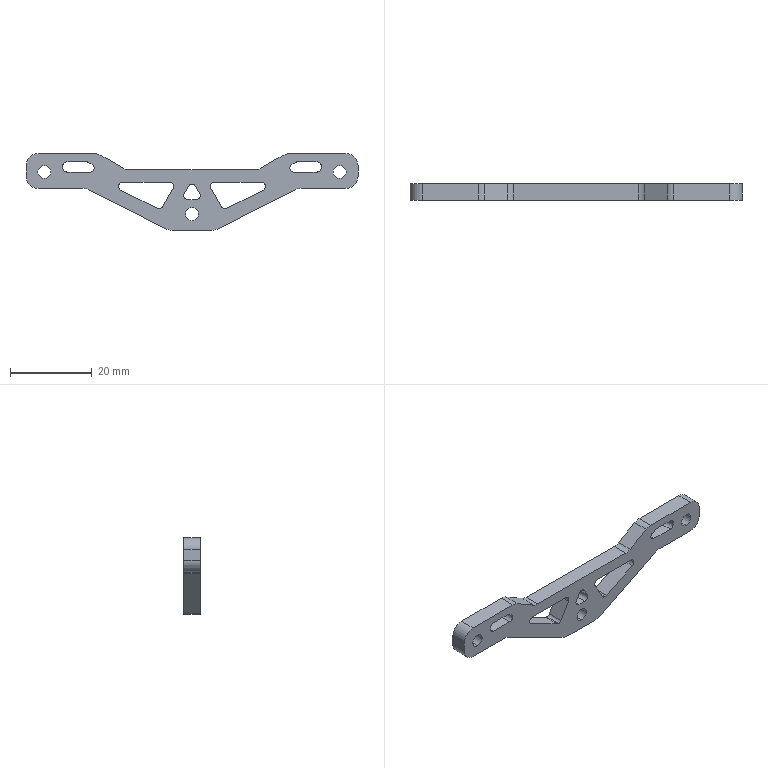Part | SolidWorks | features Fillet 2, Extrusion 1, ICE 1 | 1 solid | 68 faces | box 81 x 4 x 18.75 mm | volume 2669 mm3 | cylinder 37 | plane 31 | commonest cylinder face diameters 2 x19 6 x12 3.2 x6